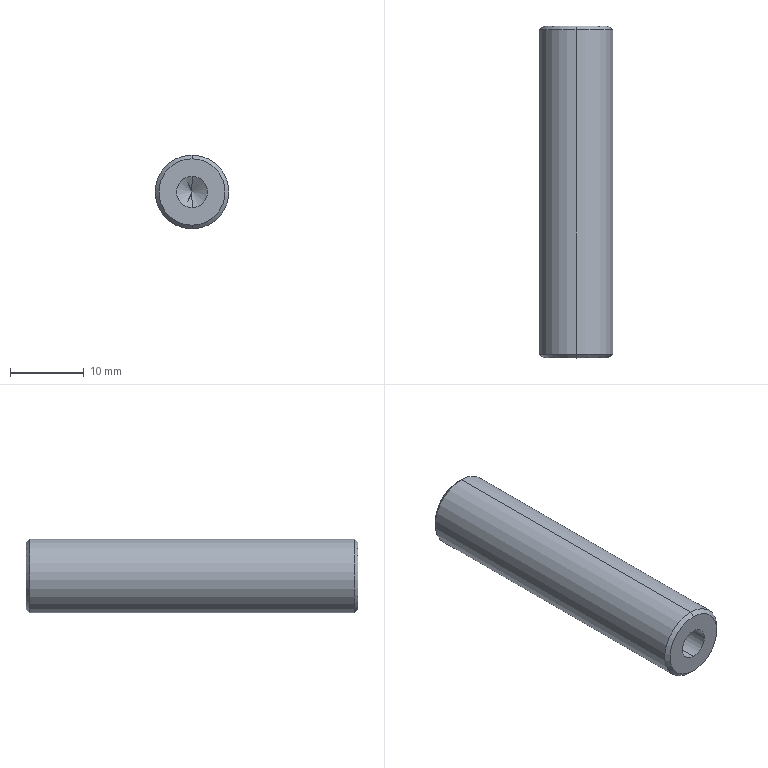Part | SolidWorks | features 3DProfileFeature 1, Chamfer 1, Extrusion 1, HoleWzd 1 | 1 solid | 12 faces | box 10 x 45 x 10 mm | volume 3349 mm3 | cone 6 | cylinder 4 | plane 2 | commonest cylinder face diameters 4.2 x2 10 x2
STEP:
#1=CARTESIAN_POINT('',(0.,45.,4.5));
#2=VERTEX_POINT('',#1);
#3=CARTESIAN_POINT('',(0.,45.,-4.5));
#4=VERTEX_POINT('',#3);
#5=CARTESIAN_POINT('',(0.,45.,0.));
#6=DIRECTION('',(0.,1.,0.));
#7=DIRECTION('',(0.,0.,1.));
#8=AXIS2_PLACEMENT_3D('',#5,#6,#7);
#9=CIRCLE('',#8,4.5);
#10=EDGE_CURVE('',#2,#4,#9,.T.);
#11=ORIENTED_EDGE('',*,*,#10,.F.);
#12=CARTESIAN_POINT('',(0.,44.5,5.));
#13=VERTEX_POINT('',#12);
#14=CARTESIAN_POINT('',(0.,45.,4.5));
#15=DIRECTION('',(0.,-0.7071,0.7071));
#16=VECTOR('',#15,1000.);
#17=LINE('',#14,#16);
#18=EDGE_CURVE('',#2,#13,#17,.T.);
#19=ORIENTED_EDGE('',*,*,#18,.T.);
#20=CARTESIAN_POINT('',(0.,44.5,-5.));
#21=VERTEX_POINT('',#20);
#22=CARTESIAN_POINT('',(0.,44.5,0.));
#23=DIRECTION('',(0.,-1.,0.));
#24=DIRECTION('',(0.,0.,1.));
#25=AXIS2_PLACEMENT_3D('',#22,#23,#24);
#26=CIRCLE('',#25,5.);
#27=EDGE_CURVE('',#21,#13,#26,.T.);
#28=ORIENTED_EDGE('',*,*,#27,.F.);
#29=CARTESIAN_POINT('',(0.,45.,-4.5));
#30=DIRECTION('',(0.,-0.7071,-0.7071));
#31=VECTOR('',#30,1000.);
#32=LINE('',#29,#31);
#33=EDGE_CURVE('',#4,#21,#32,.T.);
#34=ORIENTED_EDGE('',*,*,#33,.F.);
#35=EDGE_LOOP('',(#11,#19,#28,#34));
#36=FACE_OUTER_BOUND('',#35,.T.);
#37=CARTESIAN_POINT('',(0.,45.,0.));
#38=DIRECTION('',(0.,-1.,0.));
#39=DIRECTION('',(0.,0.,-1.));
#40=AXIS2_PLACEMENT_3D('',#37,#38,#39);
#41=CONICAL_SURFACE('',#40,4.5,0.7854);
#42=ADVANCED_FACE('',(#36),#41,.T.);
#43=CARTESIAN_POINT('',(0.,0.,-4.5));
#44=VERTEX_POINT('',#43);
#45=CARTESIAN_POINT('',(0.,0.,4.5));
#46=VERTEX_POINT('',#45);
#47=CARTESIAN_POINT('',(0.,0.,0.));
#48=DIRECTION('',(0.,-1.,0.));
#49=DIRECTION('',(0.,0.,1.));
#50=AXIS2_PLACEMENT_3D('',#47,#48,#49);
#51=CIRCLE('',#50,4.5);
#52=EDGE_CURVE('',#44,#46,#51,.T.);
#53=ORIENTED_EDGE('',*,*,#52,.F.);
#54=CARTESIAN_POINT('',(0.,0.5,-5.));
#55=VERTEX_POINT('',#54);
#56=CARTESIAN_POINT('',(0.,0.5,-5.));
#57=DIRECTION('',(0.,0.7071,-0.7071));
#58=VECTOR('',#57,1000.);
#59=LINE('',#56,#58);
#60=EDGE_CURVE('',#44,#55,#59,.T.);
#61=ORIENTED_EDGE('',*,*,#60,.T.);
#62=CARTESIAN_POINT('',(0.,0.5,5.));
#63=VERTEX_POINT('',#62);
#64=CARTESIAN_POINT('',(0.,0.5,0.));
#65=DIRECTION('',(0.,1.,0.));
#66=DIRECTION('',(0.,0.,1.));
#67=AXIS2_PLACEMENT_3D('',#64,#65,#66);
#68=CIRCLE('',#67,5.);
#69=EDGE_CURVE('',#63,#55,#68,.T.);
#70=ORIENTED_EDGE('',*,*,#69,.F.);
#71=CARTESIAN_POINT('',(0.,0.5,5.));
#72=DIRECTION('',(0.,0.7071,0.7071));
#73=VECTOR('',#72,1000.);
#74=LINE('',#71,#73);
#75=EDGE_CURVE('',#46,#63,#74,.T.);
#76=ORIENTED_EDGE('',*,*,#75,.F.);
#77=EDGE_LOOP('',(#53,#61,#70,#76));
#78=FACE_OUTER_BOUND('',#77,.T.);
#79=CARTESIAN_POINT('',(0.,0.5,0.));
#80=DIRECTION('',(0.,1.,0.));
#81=DIRECTION('',(0.,0.,1.));
#82=AXIS2_PLACEMENT_3D('',#79,#80,#81);
#83=CONICAL_SURFACE('',#82,5.,0.7854);
#84=ADVANCED_FACE('',(#78),#83,.T.);
#85=CARTESIAN_POINT('',(0.,12.4,2.1));
#86=VERTEX_POINT('',#85);
#87=CARTESIAN_POINT('',(0.,12.4,-2.1));
#88=VERTEX_POINT('',#87);
#89=CARTESIAN_POINT('',(0.,12.4,0.));
#90=DIRECTION('',(0.,-1.,0.));
#91=DIRECTION('',(0.,0.,-1.));
#92=AXIS2_PLACEMENT_3D('',#89,#90,#91);
#93=CIRCLE('',#92,2.1);
#94=EDGE_CURVE('',#86,#88,#93,.T.);
#95=ORIENTED_EDGE('',*,*,#94,.F.);
#96=CARTESIAN_POINT('',(0.,0.,2.1));
#97=VERTEX_POINT('',#96);
#98=CARTESIAN_POINT('',(0.,0.,2.1));
#99=DIRECTION('',(0.,-1.,0.));
#100=VECTOR('',#99,1000.);
#101=LINE('',#98,#100);
#102=EDGE_CURVE('',#86,#97,#101,.T.);
#103=ORIENTED_EDGE('',*,*,#102,.T.);
#104=CARTESIAN_POINT('',(0.,0.,-2.1));
#105=VERTEX_POINT('',#104);
#106=CARTESIAN_POINT('',(0.,0.,0.));
#107=DIRECTION('',(0.,-1.,0.));
#108=DIRECTION('',(0.,0.,-1.));
#109=AXIS2_PLACEMENT_3D('',#106,#107,#108);
#110=CIRCLE('',#109,2.1);
#111=EDGE_CURVE('',#97,#105,#110,.T.);
#112=ORIENTED_EDGE('',*,*,#111,.T.);
#113=CARTESIAN_POINT('',(0.,0.,-2.1));
#114=DIRECTION('',(0.,-1.,0.));
#115=VECTOR('',#114,1000.);
#116=LINE('',#113,#115);
#117=EDGE_CURVE('',#88,#105,#116,.T.);
#118=ORIENTED_EDGE('',*,*,#117,.F.);
#119=EDGE_LOOP('',(#95,#103,#112,#118));
#120=FACE_OUTER_BOUND('',#119,.T.);
#121=CARTESIAN_POINT('',(0.,0.,0.));
#122=DIRECTION('',(0.,-1.,0.));
#123=DIRECTION('',(0.,0.,-1.));
#124=AXIS2_PLACEMENT_3D('',#121,#122,#123);
#125=CYLINDRICAL_SURFACE('',#124,2.1);
#126=ADVANCED_FACE('',(#120),#125,.F.);
#127=CARTESIAN_POINT('',(0.,13.662,0.));
#128=VERTEX_POINT('',#127);
#129=CARTESIAN_POINT('',(0.,12.4,-2.1));
#130=DIRECTION('',(0.,-0.515,-0.8572));
#131=VECTOR('',#130,1000.);
#132=LINE('',#129,#131);
#133=EDGE_CURVE('',#128,#88,#132,.T.);
#134=ORIENTED_EDGE('',*,*,#133,.F.);
#135=CARTESIAN_POINT('',(0.,12.4,2.1));
#136=DIRECTION('',(0.,-0.515,0.8572));
#137=VECTOR('',#136,1000.);
#138=LINE('',#135,#137);
#139=EDGE_CURVE('',#128,#86,#138,.T.);
#140=ORIENTED_EDGE('',*,*,#139,.T.);
#141=ORIENTED_EDGE('',*,*,#94,.T.);
#142=EDGE_LOOP('',(#134,#140,#141));
#143=FACE_OUTER_BOUND('',#142,.T.);
#144=CARTESIAN_POINT('',(0.,12.4,0.));
#145=DIRECTION('',(0.,-1.,0.));
#146=DIRECTION('',(0.,0.,-1.));
#147=AXIS2_PLACEMENT_3D('',#144,#145,#146);
#148=CONICAL_SURFACE('',#147,2.1,1.03);
#149=ADVANCED_FACE('',(#143),#148,.F.);
#150=ORIENTED_EDGE('',*,*,#27,.T.);
#151=CARTESIAN_POINT('',(0.,45.,5.));
#152=DIRECTION('',(0.,-1.,0.));
#153=VECTOR('',#152,1000.);
#154=LINE('',#151,#153);
#155=EDGE_CURVE('',#13,#63,#154,.T.);
#156=ORIENTED_EDGE('',*,*,#155,.T.);
#157=ORIENTED_EDGE('',*,*,#69,.T.);
#158=CARTESIAN_POINT('',(0.,45.,-5.));
#159=DIRECTION('',(0.,-1.,0.));
#160=VECTOR('',#159,1000.);
#161=LINE('',#158,#160);
#162=EDGE_CURVE('',#21,#55,#161,.T.);
#163=ORIENTED_EDGE('',*,*,#162,.F.);
#164=EDGE_LOOP('',(#150,#156,#157,#163));
#165=FACE_OUTER_BOUND('',#164,.T.);
#166=CARTESIAN_POINT('',(0.,45.,0.));
#167=DIRECTION('',(0.,-1.,0.));
#168=DIRECTION('',(0.,0.,-1.));
#169=AXIS2_PLACEMENT_3D('',#166,#167,#168);
#170=CYLINDRICAL_SURFACE('',#169,5.);
#171=ADVANCED_FACE('',(#165),#170,.T.);
#172=CARTESIAN_POINT('',(0.,0.,0.));
#173=DIRECTION('',(0.,-1.,0.));
#174=DIRECTION('',(0.,0.,1.));
#175=AXIS2_PLACEMENT_3D('',#172,#173,#174);
#176=CIRCLE('',#175,4.5);
#177=EDGE_CURVE('',#46,#44,#176,.T.);
#178=ORIENTED_EDGE('',*,*,#177,.T.);
#179=ORIENTED_EDGE('',*,*,#52,.T.);
#180=EDGE_LOOP('',(#178,#179));
#181=FACE_OUTER_BOUND('',#180,.T.);
#182=CARTESIAN_POINT('',(0.,0.,0.));
#183=DIRECTION('',(0.,-1.,0.));
#184=DIRECTION('',(0.,0.,-1.));
#185=AXIS2_PLACEMENT_3D('',#182,#183,#184);
#186=CIRCLE('',#185,2.1);
#187=EDGE_CURVE('',#105,#97,#186,.T.);
#188=ORIENTED_EDGE('',*,*,#187,.F.);
#189=ORIENTED_EDGE('',*,*,#111,.F.);
#190=EDGE_LOOP('',(#188,#189));
#191=FACE_BOUND('',#190,.T.);
#192=CARTESIAN_POINT('',(0.,0.,0.));
#193=DIRECTION('',(0.,1.,0.));
#194=DIRECTION('',(0.,0.,1.));
#195=AXIS2_PLACEMENT_3D('',#192,#193,#194);
#196=PLANE('',#195);
#197=ADVANCED_FACE('',(#181,#191),#196,.F.);
#198=ORIENTED_EDGE('',*,*,#155,.F.);
#199=CARTESIAN_POINT('',(0.,44.5,0.));
#200=DIRECTION('',(0.,-1.,0.));
#201=DIRECTION('',(0.,0.,1.));
#202=AXIS2_PLACEMENT_3D('',#199,#200,#201);
#203=CIRCLE('',#202,5.);
#204=EDGE_CURVE('',#13,#21,#203,.T.);
#205=ORIENTED_EDGE('',*,*,#204,.T.);
#206=ORIENTED_EDGE('',*,*,#162,.T.);
#207=CARTESIAN_POINT('',(0.,0.5,0.));
#208=DIRECTION('',(0.,1.,0.));
#209=DIRECTION('',(0.,0.,1.));
#210=AXIS2_PLACEMENT_3D('',#207,#208,#209);
#211=CIRCLE('',#210,5.);
#212=EDGE_CURVE('',#55,#63,#211,.T.);
#213=ORIENTED_EDGE('',*,*,#212,.T.);
#214=EDGE_LOOP('',(#198,#205,#206,#213));
#215=FACE_OUTER_BOUND('',#214,.T.);
#216=CARTESIAN_POINT('',(0.,45.,0.));
#217=DIRECTION('',(0.,-1.,0.));
#218=DIRECTION('',(0.,0.,-1.));
#219=AXIS2_PLACEMENT_3D('',#216,#217,#218);
#220=CYLINDRICAL_SURFACE('',#219,5.);
#221=ADVANCED_FACE('',(#215),#220,.T.);
#222=CARTESIAN_POINT('',(0.,45.,0.));
#223=DIRECTION('',(0.,1.,0.));
#224=DIRECTION('',(0.,0.,1.));
#225=AXIS2_PLACEMENT_3D('',#222,#223,#224);
#226=CIRCLE('',#225,4.5);
#227=EDGE_CURVE('',#4,#2,#226,.T.);
#228=ORIENTED_EDGE('',*,*,#227,.T.);
#229=ORIENTED_EDGE('',*,*,#10,.T.);
#230=EDGE_LOOP('',(#228,#229));
#231=FACE_OUTER_BOUND('',#230,.T.);
#232=CARTESIAN_POINT('',(0.,45.,0.));
#233=DIRECTION('',(0.,1.,0.));
#234=DIRECTION('',(0.,0.,1.));
#235=AXIS2_PLACEMENT_3D('',#232,#233,#234);
#236=PLANE('',#235);
#237=ADVANCED_FACE('',(#231),#236,.T.);
#238=ORIENTED_EDGE('',*,*,#139,.F.);
#239=ORIENTED_EDGE('',*,*,#133,.T.);
#240=CARTESIAN_POINT('',(0.,12.4,0.));
#241=DIRECTION('',(0.,-1.,0.));
#242=DIRECTION('',(0.,0.,-1.));
#243=AXIS2_PLACEMENT_3D('',#240,#241,#242);
#244=CIRCLE('',#243,2.1);
#245=EDGE_CURVE('',#88,#86,#244,.T.);
#246=ORIENTED_EDGE('',*,*,#245,.T.);
#247=EDGE_LOOP('',(#238,#239,#246));
#248=FACE_OUTER_BOUND('',#247,.T.);
#249=CARTESIAN_POINT('',(0.,12.4,0.));
#250=DIRECTION('',(0.,-1.,0.));
#251=DIRECTION('',(0.,0.,-1.));
#252=AXIS2_PLACEMENT_3D('',#249,#250,#251);
#253=CONICAL_SURFACE('',#252,2.1,1.03);
#254=ADVANCED_FACE('',(#248),#253,.F.);
#255=ORIENTED_EDGE('',*,*,#102,.F.);
#256=ORIENTED_EDGE('',*,*,#245,.F.);
#257=ORIENTED_EDGE('',*,*,#117,.T.);
#258=ORIENTED_EDGE('',*,*,#187,.T.);
#259=EDGE_LOOP('',(#255,#256,#257,#258));
#260=FACE_OUTER_BOUND('',#259,.T.);
#261=CARTESIAN_POINT('',(0.,0.,0.));
#262=DIRECTION('',(0.,-1.,0.));
#263=DIRECTION('',(0.,0.,-1.));
#264=AXIS2_PLACEMENT_3D('',#261,#262,#263);
#265=CYLINDRICAL_SURFACE('',#264,2.1);
#266=ADVANCED_FACE('',(#260),#265,.F.);
#267=ORIENTED_EDGE('',*,*,#60,.F.);
#268=ORIENTED_EDGE('',*,*,#177,.F.);
#269=ORIENTED_EDGE('',*,*,#75,.T.);
#270=ORIENTED_EDGE('',*,*,#212,.F.);
#271=EDGE_LOOP('',(#267,#268,#269,#270));
#272=FACE_OUTER_BOUND('',#271,.T.);
#273=CARTESIAN_POINT('',(0.,0.5,0.));
#274=DIRECTION('',(0.,1.,0.));
#275=DIRECTION('',(0.,0.,1.));
#276=AXIS2_PLACEMENT_3D('',#273,#274,#275);
#277=CONICAL_SURFACE('',#276,5.,0.7854);
#278=ADVANCED_FACE('',(#272),#277,.T.);
#279=ORIENTED_EDGE('',*,*,#18,.F.);
#280=ORIENTED_EDGE('',*,*,#227,.F.);
#281=ORIENTED_EDGE('',*,*,#33,.T.);
#282=ORIENTED_EDGE('',*,*,#204,.F.);
#283=EDGE_LOOP('',(#279,#280,#281,#282));
#284=FACE_OUTER_BOUND('',#283,.T.);
#285=CARTESIAN_POINT('',(0.,45.,0.));
#286=DIRECTION('',(0.,-1.,0.));
#287=DIRECTION('',(0.,0.,-1.));
#288=AXIS2_PLACEMENT_3D('',#285,#286,#287);
#289=CONICAL_SURFACE('',#288,4.5,0.7854);
#290=ADVANCED_FACE('',(#284),#289,.T.);
#291=CLOSED_SHELL('',(#42,#84,#126,#149,#171,#197,#221,#237,#254,#266,#278,#290));
#292=MANIFOLD_SOLID_BREP('',#291);
#293=CARTESIAN_POINT('',(0.,0.,0.));
#294=DIRECTION('',(0.,0.,1.));
#295=DIRECTION('',(1.,0.,0.));
#296=AXIS2_PLACEMENT_3D('',#293,#294,#295);
#297=(LENGTH_UNIT()NAMED_UNIT(*)SI_UNIT(.MILLI.,.METRE.));
#298=UNCERTAINTY_MEASURE_WITH_UNIT(LENGTH_MEASURE(0.00001),#297,'','');
#299=(NAMED_UNIT(*)PLANE_ANGLE_UNIT()SI_UNIT($,.RADIAN.));
#300=(NAMED_UNIT(*)SI_UNIT($,.STERADIAN.)SOLID_ANGLE_UNIT());
#301=(GEOMETRIC_REPRESENTATION_CONTEXT(3)GLOBAL_UNCERTAINTY_ASSIGNED_CONTEXT((#298))GLOBAL_UNIT_ASSIGNED_CONTEXT((#297,#299,#300))REPRESENTATION_CONTEXT('',''));
#302=ADVANCED_BREP_SHAPE_REPRESENTATION('',(#292,#296),#301);